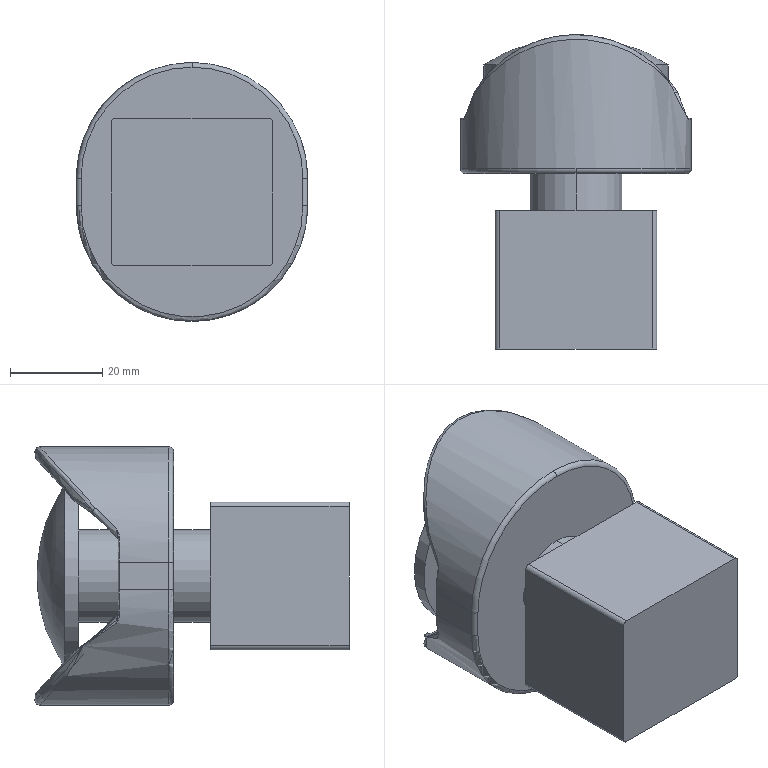Part | STEP file | Component | 1 solid | 93 faces | box 50 x 68 x 56 mm | volume 64949 mm3 | spline 43 | cylinder 32 | plane 15 | torus 3 | commonest cylinder face diameters 0.6 x8 2 x6 20 x4 75.358 x4 44 x3 50 x3